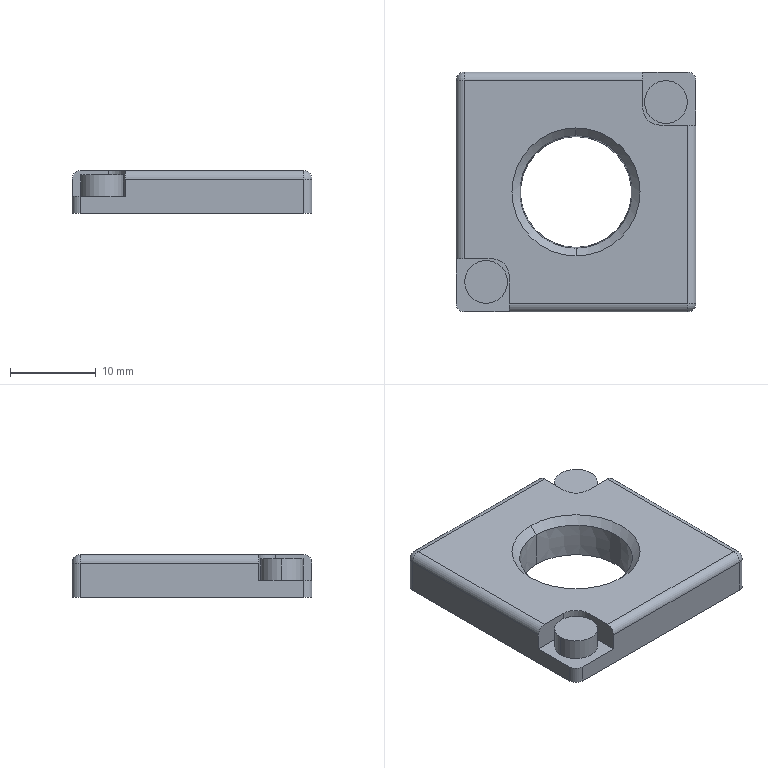Part | STEP file | AC40-04-KSTV-38JNR_AC3009A Gauge-2 | 1 solid | 34 faces | box 28 x 28 x 5 mm | volume 3081 mm3 | cylinder 14 | plane 14 | cone 4 | sphere 2 | commonest cylinder face diameters 2 x8 5 x4 4 x2